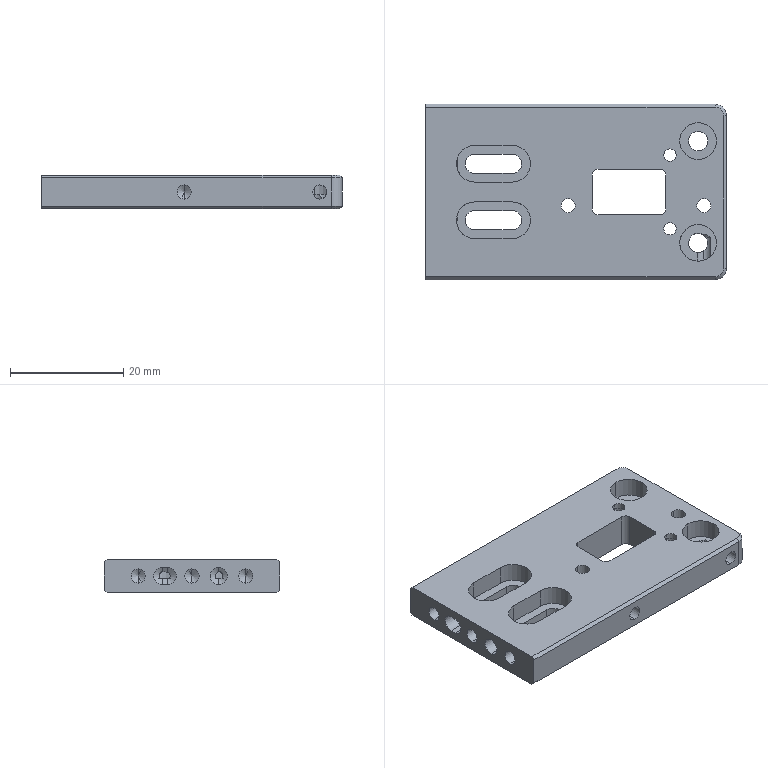Part | 1 solid | 100 faces | box 53.2 x 31 x 6 mm | volume 7878 mm3 | cylinder 48 | plane 34 | cone 18 | commonest cylinder face diameters 2.5 x14 3 x8 3.4 x8 6.5 x8 2 x4 2.2 x4